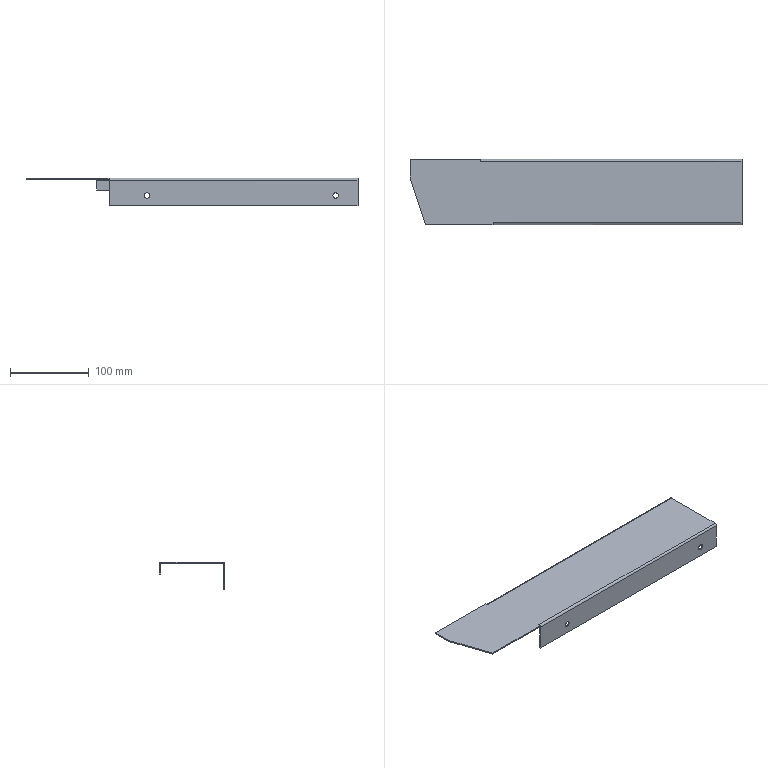Part | STEP file | Top flange baffle 2 | 1 solid | 31 faces | box 422.83 x 83 x 35 mm | volume 73586 mm3 | plane 23 | cylinder 8 | commonest cylinder face diameters 7 x4 2 x2 5 x2